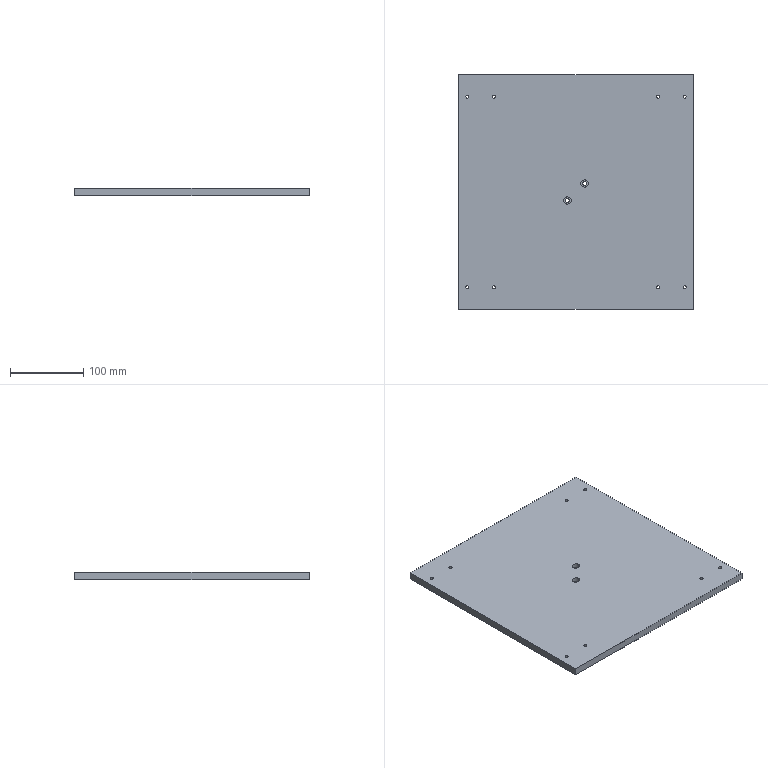Part | SolidWorks | features HoleWzd 2, MirrorPattern 2, Extrusion 1 | 1 solid | 32 faces | box 320 x 320 x 10 mm | volume 1021792 mm3 | cylinder 24 | plane 8 | commonest cylinder face diameters 4.2 x16 5.5 x4 10 x4
STEP:
#1=CARTESIAN_POINT('',(-145.9,-130.,10.));
#2=VERTEX_POINT('',#1);
#3=CARTESIAN_POINT('',(-150.1,-130.,10.));
#4=VERTEX_POINT('',#3);
#5=CARTESIAN_POINT('',(-148.,-130.,10.));
#6=DIRECTION('',(0.,0.,-1.));
#7=DIRECTION('',(-1.,0.,0.));
#8=AXIS2_PLACEMENT_3D('',#5,#6,#7);
#9=CIRCLE('',#8,2.1);
#10=EDGE_CURVE('',#2,#4,#9,.T.);
#11=ORIENTED_EDGE('',*,*,#10,.F.);
#12=CARTESIAN_POINT('',(-145.9,-130.,0.));
#13=VERTEX_POINT('',#12);
#14=CARTESIAN_POINT('',(-145.9,-130.,0.));
#15=DIRECTION('',(0.,0.,-1.));
#16=VECTOR('',#15,1000.);
#17=LINE('',#14,#16);
#18=EDGE_CURVE('',#2,#13,#17,.T.);
#19=ORIENTED_EDGE('',*,*,#18,.T.);
#20=CARTESIAN_POINT('',(-150.1,-130.,0.));
#21=VERTEX_POINT('',#20);
#22=CARTESIAN_POINT('',(-148.,-130.,0.));
#23=DIRECTION('',(0.,0.,-1.));
#24=DIRECTION('',(-1.,0.,0.));
#25=AXIS2_PLACEMENT_3D('',#22,#23,#24);
#26=CIRCLE('',#25,2.1);
#27=EDGE_CURVE('',#13,#21,#26,.T.);
#28=ORIENTED_EDGE('',*,*,#27,.T.);
#29=CARTESIAN_POINT('',(-150.1,-130.,0.));
#30=DIRECTION('',(0.,0.,-1.));
#31=VECTOR('',#30,1000.);
#32=LINE('',#29,#31);
#33=EDGE_CURVE('',#4,#21,#32,.T.);
#34=ORIENTED_EDGE('',*,*,#33,.F.);
#35=EDGE_LOOP('',(#11,#19,#28,#34));
#36=FACE_OUTER_BOUND('',#35,.T.);
#37=CARTESIAN_POINT('',(-148.,-130.,0.));
#38=DIRECTION('',(0.,0.,-1.));
#39=DIRECTION('',(-1.,0.,0.));
#40=AXIS2_PLACEMENT_3D('',#37,#38,#39);
#41=CYLINDRICAL_SURFACE('',#40,2.1);
#42=ADVANCED_FACE('',(#36),#41,.F.);
#43=CARTESIAN_POINT('',(-109.9,-130.,10.));
#44=VERTEX_POINT('',#43);
#45=CARTESIAN_POINT('',(-114.1,-130.,10.));
#46=VERTEX_POINT('',#45);
#47=CARTESIAN_POINT('',(-112.,-130.,10.));
#48=DIRECTION('',(0.,0.,-1.));
#49=DIRECTION('',(-1.,0.,0.));
#50=AXIS2_PLACEMENT_3D('',#47,#48,#49);
#51=CIRCLE('',#50,2.1);
#52=EDGE_CURVE('',#44,#46,#51,.T.);
#53=ORIENTED_EDGE('',*,*,#52,.F.);
#54=CARTESIAN_POINT('',(-109.9,-130.,0.));
#55=VERTEX_POINT('',#54);
#56=CARTESIAN_POINT('',(-109.9,-130.,0.));
#57=DIRECTION('',(0.,0.,-1.));
#58=VECTOR('',#57,1000.);
#59=LINE('',#56,#58);
#60=EDGE_CURVE('',#44,#55,#59,.T.);
#61=ORIENTED_EDGE('',*,*,#60,.T.);
#62=CARTESIAN_POINT('',(-114.1,-130.,0.));
#63=VERTEX_POINT('',#62);
#64=CARTESIAN_POINT('',(-112.,-130.,0.));
#65=DIRECTION('',(0.,0.,-1.));
#66=DIRECTION('',(-1.,0.,0.));
#67=AXIS2_PLACEMENT_3D('',#64,#65,#66);
#68=CIRCLE('',#67,2.1);
#69=EDGE_CURVE('',#55,#63,#68,.T.);
#70=ORIENTED_EDGE('',*,*,#69,.T.);
#71=CARTESIAN_POINT('',(-114.1,-130.,0.));
#72=DIRECTION('',(0.,0.,-1.));
#73=VECTOR('',#72,1000.);
#74=LINE('',#71,#73);
#75=EDGE_CURVE('',#46,#63,#74,.T.);
#76=ORIENTED_EDGE('',*,*,#75,.F.);
#77=EDGE_LOOP('',(#53,#61,#70,#76));
#78=FACE_OUTER_BOUND('',#77,.T.);
#79=CARTESIAN_POINT('',(-112.,-130.,0.));
#80=DIRECTION('',(0.,0.,-1.));
#81=DIRECTION('',(-1.,0.,0.));
#82=AXIS2_PLACEMENT_3D('',#79,#80,#81);
#83=CYLINDRICAL_SURFACE('',#82,2.1);
#84=ADVANCED_FACE('',(#78),#83,.F.);
#85=CARTESIAN_POINT('',(-145.9,130.,10.));
#86=VERTEX_POINT('',#85);
#87=CARTESIAN_POINT('',(-150.1,130.,10.));
#88=VERTEX_POINT('',#87);
#89=CARTESIAN_POINT('',(-148.,130.,10.));
#90=DIRECTION('',(0.,0.,-1.));
#91=DIRECTION('',(-1.,0.,0.));
#92=AXIS2_PLACEMENT_3D('',#89,#90,#91);
#93=CIRCLE('',#92,2.1);
#94=EDGE_CURVE('',#86,#88,#93,.T.);
#95=ORIENTED_EDGE('',*,*,#94,.F.);
#96=CARTESIAN_POINT('',(-145.9,130.,0.));
#97=VERTEX_POINT('',#96);
#98=CARTESIAN_POINT('',(-145.9,130.,0.));
#99=DIRECTION('',(0.,0.,-1.));
#100=VECTOR('',#99,1000.);
#101=LINE('',#98,#100);
#102=EDGE_CURVE('',#86,#97,#101,.T.);
#103=ORIENTED_EDGE('',*,*,#102,.T.);
#104=CARTESIAN_POINT('',(-150.1,130.,0.));
#105=VERTEX_POINT('',#104);
#106=CARTESIAN_POINT('',(-148.,130.,0.));
#107=DIRECTION('',(0.,0.,-1.));
#108=DIRECTION('',(-1.,0.,0.));
#109=AXIS2_PLACEMENT_3D('',#106,#107,#108);
#110=CIRCLE('',#109,2.1);
#111=EDGE_CURVE('',#97,#105,#110,.T.);
#112=ORIENTED_EDGE('',*,*,#111,.T.);
#113=CARTESIAN_POINT('',(-150.1,130.,0.));
#114=DIRECTION('',(0.,0.,-1.));
#115=VECTOR('',#114,1000.);
#116=LINE('',#113,#115);
#117=EDGE_CURVE('',#88,#105,#116,.T.);
#118=ORIENTED_EDGE('',*,*,#117,.F.);
#119=EDGE_LOOP('',(#95,#103,#112,#118));
#120=FACE_OUTER_BOUND('',#119,.T.);
#121=CARTESIAN_POINT('',(-148.,130.,0.));
#122=DIRECTION('',(0.,0.,-1.));
#123=DIRECTION('',(-1.,0.,0.));
#124=AXIS2_PLACEMENT_3D('',#121,#122,#123);
#125=CYLINDRICAL_SURFACE('',#124,2.1);
#126=ADVANCED_FACE('',(#120),#125,.F.);
#127=CARTESIAN_POINT('',(-109.9,130.,10.));
#128=VERTEX_POINT('',#127);
#129=CARTESIAN_POINT('',(-114.1,130.,10.));
#130=VERTEX_POINT('',#129);
#131=CARTESIAN_POINT('',(-112.,130.,10.));
#132=DIRECTION('',(0.,0.,-1.));
#133=DIRECTION('',(-1.,0.,0.));
#134=AXIS2_PLACEMENT_3D('',#131,#132,#133);
#135=CIRCLE('',#134,2.1);
#136=EDGE_CURVE('',#128,#130,#135,.T.);
#137=ORIENTED_EDGE('',*,*,#136,.F.);
#138=CARTESIAN_POINT('',(-109.9,130.,0.));
#139=VERTEX_POINT('',#138);
#140=CARTESIAN_POINT('',(-109.9,130.,0.));
#141=DIRECTION('',(0.,0.,-1.));
#142=VECTOR('',#141,1000.);
#143=LINE('',#140,#142);
#144=EDGE_CURVE('',#128,#139,#143,.T.);
#145=ORIENTED_EDGE('',*,*,#144,.T.);
#146=CARTESIAN_POINT('',(-114.1,130.,0.));
#147=VERTEX_POINT('',#146);
#148=CARTESIAN_POINT('',(-112.,130.,0.));
#149=DIRECTION('',(0.,0.,-1.));
#150=DIRECTION('',(-1.,0.,0.));
#151=AXIS2_PLACEMENT_3D('',#148,#149,#150);
#152=CIRCLE('',#151,2.1);
#153=EDGE_CURVE('',#139,#147,#152,.T.);
#154=ORIENTED_EDGE('',*,*,#153,.T.);
#155=CARTESIAN_POINT('',(-114.1,130.,0.));
#156=DIRECTION('',(0.,0.,-1.));
#157=VECTOR('',#156,1000.);
#158=LINE('',#155,#157);
#159=EDGE_CURVE('',#130,#147,#158,.T.);
#160=ORIENTED_EDGE('',*,*,#159,.F.);
#161=EDGE_LOOP('',(#137,#145,#154,#160));
#162=FACE_OUTER_BOUND('',#161,.T.);
#163=CARTESIAN_POINT('',(-112.,130.,0.));
#164=DIRECTION('',(0.,0.,-1.));
#165=DIRECTION('',(-1.,0.,0.));
#166=AXIS2_PLACEMENT_3D('',#163,#164,#165);
#167=CYLINDRICAL_SURFACE('',#166,2.1);
#168=ADVANCED_FACE('',(#162),#167,.F.);
#169=CARTESIAN_POINT('',(150.1,-130.,10.));
#170=VERTEX_POINT('',#169);
#171=CARTESIAN_POINT('',(145.9,-130.,10.));
#172=VERTEX_POINT('',#171);
#173=CARTESIAN_POINT('',(148.,-130.,10.));
#174=DIRECTION('',(0.,0.,-1.));
#175=DIRECTION('',(-1.,0.,0.));
#176=AXIS2_PLACEMENT_3D('',#173,#174,#175);
#177=CIRCLE('',#176,2.1);
#178=EDGE_CURVE('',#170,#172,#177,.T.);
#179=ORIENTED_EDGE('',*,*,#178,.F.);
#180=CARTESIAN_POINT('',(150.1,-130.,0.));
#181=VERTEX_POINT('',#180);
#182=CARTESIAN_POINT('',(150.1,-130.,0.));
#183=DIRECTION('',(0.,0.,-1.));
#184=VECTOR('',#183,1000.);
#185=LINE('',#182,#184);
#186=EDGE_CURVE('',#170,#181,#185,.T.);
#187=ORIENTED_EDGE('',*,*,#186,.T.);
#188=CARTESIAN_POINT('',(145.9,-130.,0.));
#189=VERTEX_POINT('',#188);
#190=CARTESIAN_POINT('',(148.,-130.,0.));
#191=DIRECTION('',(0.,0.,-1.));
#192=DIRECTION('',(-1.,0.,0.));
#193=AXIS2_PLACEMENT_3D('',#190,#191,#192);
#194=CIRCLE('',#193,2.1);
#195=EDGE_CURVE('',#181,#189,#194,.T.);
#196=ORIENTED_EDGE('',*,*,#195,.T.);
#197=CARTESIAN_POINT('',(145.9,-130.,0.));
#198=DIRECTION('',(0.,0.,-1.));
#199=VECTOR('',#198,1000.);
#200=LINE('',#197,#199);
#201=EDGE_CURVE('',#172,#189,#200,.T.);
#202=ORIENTED_EDGE('',*,*,#201,.F.);
#203=EDGE_LOOP('',(#179,#187,#196,#202));
#204=FACE_OUTER_BOUND('',#203,.T.);
#205=CARTESIAN_POINT('',(148.,-130.,0.));
#206=DIRECTION('',(0.,0.,-1.));
#207=DIRECTION('',(-1.,0.,0.));
#208=AXIS2_PLACEMENT_3D('',#205,#206,#207);
#209=CYLINDRICAL_SURFACE('',#208,2.1);
#210=ADVANCED_FACE('',(#204),#209,.F.);
#211=CARTESIAN_POINT('',(114.1,-130.,10.));
#212=VERTEX_POINT('',#211);
#213=CARTESIAN_POINT('',(109.9,-130.,10.));
#214=VERTEX_POINT('',#213);
#215=CARTESIAN_POINT('',(112.,-130.,10.));
#216=DIRECTION('',(0.,0.,-1.));
#217=DIRECTION('',(-1.,0.,0.));
#218=AXIS2_PLACEMENT_3D('',#215,#216,#217);
#219=CIRCLE('',#218,2.1);
#220=EDGE_CURVE('',#212,#214,#219,.T.);
#221=ORIENTED_EDGE('',*,*,#220,.F.);
#222=CARTESIAN_POINT('',(114.1,-130.,0.));
#223=VERTEX_POINT('',#222);
#224=CARTESIAN_POINT('',(114.1,-130.,0.));
#225=DIRECTION('',(0.,0.,-1.));
#226=VECTOR('',#225,1000.);
#227=LINE('',#224,#226);
#228=EDGE_CURVE('',#212,#223,#227,.T.);
#229=ORIENTED_EDGE('',*,*,#228,.T.);
#230=CARTESIAN_POINT('',(109.9,-130.,0.));
#231=VERTEX_POINT('',#230);
#232=CARTESIAN_POINT('',(112.,-130.,0.));
#233=DIRECTION('',(0.,0.,-1.));
#234=DIRECTION('',(-1.,0.,0.));
#235=AXIS2_PLACEMENT_3D('',#232,#233,#234);
#236=CIRCLE('',#235,2.1);
#237=EDGE_CURVE('',#223,#231,#236,.T.);
#238=ORIENTED_EDGE('',*,*,#237,.T.);
#239=CARTESIAN_POINT('',(109.9,-130.,0.));
#240=DIRECTION('',(0.,0.,-1.));
#241=VECTOR('',#240,1000.);
#242=LINE('',#239,#241);
#243=EDGE_CURVE('',#214,#231,#242,.T.);
#244=ORIENTED_EDGE('',*,*,#243,.F.);
#245=EDGE_LOOP('',(#221,#229,#238,#244));
#246=FACE_OUTER_BOUND('',#245,.T.);
#247=CARTESIAN_POINT('',(112.,-130.,0.));
#248=DIRECTION('',(0.,0.,-1.));
#249=DIRECTION('',(-1.,0.,0.));
#250=AXIS2_PLACEMENT_3D('',#247,#248,#249);
#251=CYLINDRICAL_SURFACE('',#250,2.1);
#252=ADVANCED_FACE('',(#246),#251,.F.);
#253=CARTESIAN_POINT('',(150.1,130.,10.));
#254=VERTEX_POINT('',#253);
#255=CARTESIAN_POINT('',(145.9,130.,10.));
#256=VERTEX_POINT('',#255);
#257=CARTESIAN_POINT('',(148.,130.,10.));
#258=DIRECTION('',(0.,0.,-1.));
#259=DIRECTION('',(-1.,0.,0.));
#260=AXIS2_PLACEMENT_3D('',#257,#258,#259);
#261=CIRCLE('',#260,2.1);
#262=EDGE_CURVE('',#254,#256,#261,.T.);
#263=ORIENTED_EDGE('',*,*,#262,.F.);
#264=CARTESIAN_POINT('',(150.1,130.,0.));
#265=VERTEX_POINT('',#264);
#266=CARTESIAN_POINT('',(150.1,130.,0.));
#267=DIRECTION('',(0.,0.,-1.));
#268=VECTOR('',#267,1000.);
#269=LINE('',#266,#268);
#270=EDGE_CURVE('',#254,#265,#269,.T.);
#271=ORIENTED_EDGE('',*,*,#270,.T.);
#272=CARTESIAN_POINT('',(145.9,130.,0.));
#273=VERTEX_POINT('',#272);
#274=CARTESIAN_POINT('',(148.,130.,0.));
#275=DIRECTION('',(0.,0.,-1.));
#276=DIRECTION('',(-1.,0.,0.));
#277=AXIS2_PLACEMENT_3D('',#274,#275,#276);
#278=CIRCLE('',#277,2.1);
#279=EDGE_CURVE('',#265,#273,#278,.T.);
#280=ORIENTED_EDGE('',*,*,#279,.T.);
#281=CARTESIAN_POINT('',(145.9,130.,0.));
#282=DIRECTION('',(0.,0.,-1.));
#283=VECTOR('',#282,1000.);
#284=LINE('',#281,#283);
#285=EDGE_CURVE('',#256,#273,#284,.T.);
#286=ORIENTED_EDGE('',*,*,#285,.F.);
#287=EDGE_LOOP('',(#263,#271,#280,#286));
#288=FACE_OUTER_BOUND('',#287,.T.);
#289=CARTESIAN_POINT('',(148.,130.,0.));
#290=DIRECTION('',(0.,0.,-1.));
#291=DIRECTION('',(-1.,0.,0.));
#292=AXIS2_PLACEMENT_3D('',#289,#290,#291);
#293=CYLINDRICAL_SURFACE('',#292,2.1);
#294=ADVANCED_FACE('',(#288),#293,.F.);
#295=CARTESIAN_POINT('',(114.1,130.,10.));
#296=VERTEX_POINT('',#295);
#297=CARTESIAN_POINT('',(109.9,130.,10.));
#298=VERTEX_POINT('',#297);
#299=CARTESIAN_POINT('',(112.,130.,10.));
#300=DIRECTION('',(0.,0.,-1.));
#301=DIRECTION('',(-1.,0.,0.));
#302=AXIS2_PLACEMENT_3D('',#299,#300,#301);
#303=CIRCLE('',#302,2.1);
#304=EDGE_CURVE('',#296,#298,#303,.T.);
#305=ORIENTED_EDGE('',*,*,#304,.F.);
#306=CARTESIAN_POINT('',(114.1,130.,0.));
#307=VERTEX_POINT('',#306);
#308=CARTESIAN_POINT('',(114.1,130.,0.));
#309=DIRECTION('',(0.,0.,-1.));
#310=VECTOR('',#309,1000.);
#311=LINE('',#308,#310);
#312=EDGE_CURVE('',#296,#307,#311,.T.);
#313=ORIENTED_EDGE('',*,*,#312,.T.);
#314=CARTESIAN_POINT('',(109.9,130.,0.));
#315=VERTEX_POINT('',#314);
#316=CARTESIAN_POINT('',(112.,130.,0.));
#317=DIRECTION('',(0.,0.,-1.));
#318=DIRECTION('',(-1.,0.,0.));
#319=AXIS2_PLACEMENT_3D('',#316,#317,#318);
#320=CIRCLE('',#319,2.1);
#321=EDGE_CURVE('',#307,#315,#320,.T.);
#322=ORIENTED_EDGE('',*,*,#321,.T.);
#323=CARTESIAN_POINT('',(109.9,130.,0.));
#324=DIRECTION('',(0.,0.,-1.));
#325=VECTOR('',#324,1000.);
#326=LINE('',#323,#325);
#327=EDGE_CURVE('',#298,#315,#326,.T.);
#328=ORIENTED_EDGE('',*,*,#327,.F.);
#329=EDGE_LOOP('',(#305,#313,#322,#328));
#330=FACE_OUTER_BOUND('',#329,.T.);
#331=CARTESIAN_POINT('',(112.,130.,0.));
#332=DIRECTION('',(0.,0.,-1.));
#333=DIRECTION('',(-1.,0.,0.));
#334=AXIS2_PLACEMENT_3D('',#331,#332,#333);
#335=CYLINDRICAL_SURFACE('',#334,2.1);
#336=ADVANCED_FACE('',(#330),#335,.F.);
#337=CARTESIAN_POINT('',(-16.667,-11.667,4.3));
#338=VERTEX_POINT('',#337);
#339=CARTESIAN_POINT('',(-6.667,-11.667,4.3));
#340=VERTEX_POINT('',#339);
#341=CARTESIAN_POINT('',(-11.667,-11.667,4.3));
#342=DIRECTION('',(0.,0.,1.));
#343=DIRECTION('',(1.,0.,0.));
#344=AXIS2_PLACEMENT_3D('',#341,#342,#343);
#345=CIRCLE('',#344,5.);
#346=EDGE_CURVE('',#338,#340,#345,.T.);
#347=ORIENTED_EDGE('',*,*,#346,.F.);
#348=CARTESIAN_POINT('',(-16.667,-11.667,10.));
#349=VERTEX_POINT('',#348);
#350=CARTESIAN_POINT('',(-16.667,-11.667,10.));
#351=DIRECTION('',(0.,0.,1.));
#352=VECTOR('',#351,1000.);
#353=LINE('',#350,#352);
#354=EDGE_CURVE('',#338,#349,#353,.T.);
#355=ORIENTED_EDGE('',*,*,#354,.T.);
#356=CARTESIAN_POINT('',(-6.667,-11.667,10.));
#357=VERTEX_POINT('',#356);
#358=CARTESIAN_POINT('',(-11.667,-11.667,10.));
#359=DIRECTION('',(0.,0.,1.));
#360=DIRECTION('',(1.,0.,0.));
#361=AXIS2_PLACEMENT_3D('',#358,#359,#360);
#362=CIRCLE('',#361,5.);
#363=EDGE_CURVE('',#349,#357,#362,.T.);
#364=ORIENTED_EDGE('',*,*,#363,.T.);
#365=CARTESIAN_POINT('',(-6.667,-11.667,10.));
#366=DIRECTION('',(0.,0.,1.));
#367=VECTOR('',#366,1000.);
#368=LINE('',#365,#367);
#369=EDGE_CURVE('',#340,#357,#368,.T.);
#370=ORIENTED_EDGE('',*,*,#369,.F.);
#371=EDGE_LOOP('',(#347,#355,#364,#370));
#372=FACE_OUTER_BOUND('',#371,.T.);
#373=CARTESIAN_POINT('',(-11.667,-11.667,10.));
#374=DIRECTION('',(0.,0.,1.));
#375=DIRECTION('',(1.,0.,0.));
#376=AXIS2_PLACEMENT_3D('',#373,#374,#375);
#377=CYLINDRICAL_SURFACE('',#376,5.);
#378=ADVANCED_FACE('',(#372),#377,.F.);
#379=CARTESIAN_POINT('',(-14.417,-11.667,0.));
#380=VERTEX_POINT('',#379);
#381=CARTESIAN_POINT('',(-8.917,-11.667,0.));
#382=VERTEX_POINT('',#381);
#383=CARTESIAN_POINT('',(-11.667,-11.667,0.));
#384=DIRECTION('',(0.,0.,1.));
#385=DIRECTION('',(1.,0.,0.));
#386=AXIS2_PLACEMENT_3D('',#383,#384,#385);
#387=CIRCLE('',#386,2.75);
#388=EDGE_CURVE('',#380,#382,#387,.T.);
#389=ORIENTED_EDGE('',*,*,#388,.F.);
#390=CARTESIAN_POINT('',(-14.417,-11.667,4.3));
#391=VERTEX_POINT('',#390);
#392=CARTESIAN_POINT('',(-14.417,-11.667,10.));
#393=DIRECTION('',(0.,0.,1.));
#394=VECTOR('',#393,1000.);
#395=LINE('',#392,#394);
#396=EDGE_CURVE('',#380,#391,#395,.T.);
#397=ORIENTED_EDGE('',*,*,#396,.T.);
#398=CARTESIAN_POINT('',(-8.917,-11.667,4.3));
#399=VERTEX_POINT('',#398);
#400=CARTESIAN_POINT('',(-11.667,-11.667,4.3));
#401=DIRECTION('',(0.,0.,1.));
#402=DIRECTION('',(1.,0.,0.));
#403=AXIS2_PLACEMENT_3D('',#400,#401,#402);
#404=CIRCLE('',#403,2.75);
#405=EDGE_CURVE('',#391,#399,#404,.T.);
#406=ORIENTED_EDGE('',*,*,#405,.T.);
#407=CARTESIAN_POINT('',(-8.917,-11.667,10.));
#408=DIRECTION('',(0.,0.,1.));
#409=VECTOR('',#408,1000.);
#410=LINE('',#407,#409);
#411=EDGE_CURVE('',#382,#399,#410,.T.);
#412=ORIENTED_EDGE('',*,*,#411,.F.);
#413=EDGE_LOOP('',(#389,#397,#406,#412));
#414=FACE_OUTER_BOUND('',#413,.T.);
#415=CARTESIAN_POINT('',(-11.667,-11.667,10.));
#416=DIRECTION('',(0.,0.,1.));
#417=DIRECTION('',(1.,0.,0.));
#418=AXIS2_PLACEMENT_3D('',#415,#416,#417);
#419=CYLINDRICAL_SURFACE('',#418,2.75);
#420=ADVANCED_FACE('',(#414),#419,.F.);
#421=CARTESIAN_POINT('',(6.667,11.667,4.3));
#422=VERTEX_POINT('',#421);
#423=CARTESIAN_POINT('',(16.667,11.667,4.3));
#424=VERTEX_POINT('',#423);
#425=CARTESIAN_POINT('',(11.667,11.667,4.3));
#426=DIRECTION('',(0.,0.,1.));
#427=DIRECTION('',(1.,0.,0.));
#428=AXIS2_PLACEMENT_3D('',#425,#426,#427);
#429=CIRCLE('',#428,5.);
#430=EDGE_CURVE('',#422,#424,#429,.T.);
#431=ORIENTED_EDGE('',*,*,#430,.F.);
#432=CARTESIAN_POINT('',(6.667,11.667,10.));
#433=VERTEX_POINT('',#432);
#434=CARTESIAN_POINT('',(6.667,11.667,10.));
#435=DIRECTION('',(0.,0.,1.));
#436=VECTOR('',#435,1000.);
#437=LINE('',#434,#436);
#438=EDGE_CURVE('',#422,#433,#437,.T.);
#439=ORIENTED_EDGE('',*,*,#438,.T.);
#440=CARTESIAN_POINT('',(16.667,11.667,10.));
#441=VERTEX_POINT('',#440);
#442=CARTESIAN_POINT('',(11.667,11.667,10.));
#443=DIRECTION('',(0.,0.,1.));
#444=DIRECTION('',(1.,0.,0.));
#445=AXIS2_PLACEMENT_3D('',#442,#443,#444);
#446=CIRCLE('',#445,5.);
#447=EDGE_CURVE('',#433,#441,#446,.T.);
#448=ORIENTED_EDGE('',*,*,#447,.T.);
#449=CARTESIAN_POINT('',(16.667,11.667,10.));
#450=DIRECTION('',(0.,0.,1.));
#451=VECTOR('',#450,1000.);
#452=LINE('',#449,#451);
#453=EDGE_CURVE('',#424,#441,#452,.T.);
#454=ORIENTED_EDGE('',*,*,#453,.F.);
#455=EDGE_LOOP('',(#431,#439,#448,#454));
#456=FACE_OUTER_BOUND('',#455,.T.);
#457=CARTESIAN_POINT('',(11.667,11.667,10.));
#458=DIRECTION('',(0.,0.,1.));
#459=DIRECTION('',(1.,0.,0.));
#460=AXIS2_PLACEMENT_3D('',#457,#458,#459);
#461=CYLINDRICAL_SURFACE('',#460,5.);
#462=ADVANCED_FACE('',(#456),#461,.F.);
#463=CARTESIAN_POINT('',(8.917,11.667,0.));
#464=VERTEX_POINT('',#463);
#465=CARTESIAN_POINT('',(14.417,11.667,0.));
#466=VERTEX_POINT('',#465);
#467=CARTESIAN_POINT('',(11.667,11.667,0.));
#468=DIRECTION('',(0.,0.,1.));
#469=DIRECTION('',(1.,0.,0.));
#470=AXIS2_PLACEMENT_3D('',#467,#468,#469);
#471=CIRCLE('',#470,2.75);
#472=EDGE_CURVE('',#464,#466,#471,.T.);
#473=ORIENTED_EDGE('',*,*,#472,.F.);
#474=CARTESIAN_POINT('',(8.917,11.667,4.3));
#475=VERTEX_POINT('',#474);
#476=CARTESIAN_POINT('',(8.917,11.667,10.));
#477=DIRECTION('',(0.,0.,1.));
#478=VECTOR('',#477,1000.);
#479=LINE('',#476,#478);
#480=EDGE_CURVE('',#464,#475,#479,.T.);
#481=ORIENTED_EDGE('',*,*,#480,.T.);
#482=CARTESIAN_POINT('',(14.417,11.667,4.3));
#483=VERTEX_POINT('',#482);
#484=CARTESIAN_POINT('',(11.667,11.667,4.3));
#485=DIRECTION('',(0.,0.,1.));
#486=DIRECTION('',(1.,0.,0.));
#487=AXIS2_PLACEMENT_3D('',#484,#485,#486);
#488=CIRCLE('',#487,2.75);
#489=EDGE_CURVE('',#475,#483,#488,.T.);
#490=ORIENTED_EDGE('',*,*,#489,.T.);
#491=CARTESIAN_POINT('',(14.417,11.667,10.));
#492=DIRECTION('',(0.,0.,1.));
#493=VECTOR('',#492,1000.);
#494=LINE('',#491,#493);
#495=EDGE_CURVE('',#466,#483,#494,.T.);
#496=ORIENTED_EDGE('',*,*,#495,.F.);
#497=EDGE_LOOP('',(#473,#481,#490,#496));
#498=FACE_OUTER_BOUND('',#497,.T.);
#499=CARTESIAN_POINT('',(11.667,11.667,10.));
#500=DIRECTION('',(0.,0.,1.));
#501=DIRECTION('',(1.,0.,0.));
#502=AXIS2_PLACEMENT_3D('',#499,#500,#501);
#503=CYLINDRICAL_SURFACE('',#502,2.75);
#504=ADVANCED_FACE('',(#498),#503,.F.);
#505=CARTESIAN_POINT('',(-148.,130.,10.));
#506=DIRECTION('',(0.,0.,-1.));
#507=DIRECTION('',(-1.,0.,0.));
#508=AXIS2_PLACEMENT_3D('',#505,#506,#507);
#509=CIRCLE('',#508,2.1);
#510=EDGE_CURVE('',#88,#86,#509,.T.);
#511=ORIENTED_EDGE('',*,*,#510,.T.);
#512=ORIENTED_EDGE('',*,*,#94,.T.);
#513=EDGE_LOOP('',(#511,#512));
#514=FACE_BOUND('',#513,.T.);
#515=CARTESIAN_POINT('',(-112.,130.,10.));
#516=DIRECTION('',(0.,0.,-1.));
#517=DIRECTION('',(-1.,0.,0.));
#518=AXIS2_PLACEMENT_3D('',#515,#516,#517);
#519=CIRCLE('',#518,2.1);
#520=EDGE_CURVE('',#130,#128,#519,.T.);
#521=ORIENTED_EDGE('',*,*,#520,.T.);
#522=ORIENTED_EDGE('',*,*,#136,.T.);
#523=EDGE_LOOP('',(#521,#522));
#524=FACE_BOUND('',#523,.T.);
#525=CARTESIAN_POINT('',(160.,-160.,10.));
#526=VERTEX_POINT('',#525);
#527=CARTESIAN_POINT('',(160.,160.,10.));
#528=VERTEX_POINT('',#527);
#529=CARTESIAN_POINT('',(160.,160.,10.));
#530=DIRECTION('',(0.,1.,0.));
#531=VECTOR('',#530,1000.);
#532=LINE('',#529,#531);
#533=EDGE_CURVE('',#526,#528,#532,.T.);
#534=ORIENTED_EDGE('',*,*,#533,.T.);
#535=CARTESIAN_POINT('',(-160.,160.,10.));
#536=VERTEX_POINT('',#535);
#537=CARTESIAN_POINT('',(-160.,160.,10.));
#538=DIRECTION('',(-1.,0.,0.));
#539=VECTOR('',#538,1000.);
#540=LINE('',#537,#539);
#541=EDGE_CURVE('',#528,#536,#540,.T.);
#542=ORIENTED_EDGE('',*,*,#541,.T.);
#543=CARTESIAN_POINT('',(-160.,-160.,10.));
#544=VERTEX_POINT('',#543);
#545=CARTESIAN_POINT('',(-160.,160.,10.));
#546=DIRECTION('',(0.,-1.,0.));
#547=VECTOR('',#546,1000.);
#548=LINE('',#545,#547);
#549=EDGE_CURVE('',#536,#544,#548,.T.);
#550=ORIENTED_EDGE('',*,*,#549,.T.);
#551=CARTESIAN_POINT('',(-160.,-160.,10.));
#552=DIRECTION('',(1.,0.,0.));
#553=VECTOR('',#552,1000.);
#554=LINE('',#551,#553);
#555=EDGE_CURVE('',#544,#526,#554,.T.);
#556=ORIENTED_EDGE('',*,*,#555,.T.);
#557=EDGE_LOOP('',(#534,#542,#550,#556));
#558=FACE_OUTER_BOUND('',#557,.T.);
#559=CARTESIAN_POINT('',(11.667,11.667,10.));
#560=DIRECTION('',(0.,0.,1.));
#561=DIRECTION('',(1.,0.,0.));
#562=AXIS2_PLACEMENT_3D('',#559,#560,#561);
#563=CIRCLE('',#562,5.);
#564=EDGE_CURVE('',#441,#433,#563,.T.);
#565=ORIENTED_EDGE('',*,*,#564,.F.);
#566=ORIENTED_EDGE('',*,*,#447,.F.);
#567=EDGE_LOOP('',(#565,#566));
#568=FACE_BOUND('',#567,.T.);
#569=CARTESIAN_POINT('',(-11.667,-11.667,10.));
#570=DIRECTION('',(0.,0.,1.));
#571=DIRECTION('',(1.,0.,0.));
#572=AXIS2_PLACEMENT_3D('',#569,#570,#571);
#573=CIRCLE('',#572,5.);
#574=EDGE_CURVE('',#357,#349,#573,.T.);
#575=ORIENTED_EDGE('',*,*,#574,.F.);
#576=ORIENTED_EDGE('',*,*,#363,.F.);
#577=EDGE_LOOP('',(#575,#576));
#578=FACE_BOUND('',#577,.T.);
#579=CARTESIAN_POINT('',(112.,130.,10.));
#580=DIRECTION('',(0.,0.,-1.));
#581=DIRECTION('',(-1.,0.,0.));
#582=AXIS2_PLACEMENT_3D('',#579,#580,#581);
#583=CIRCLE('',#582,2.1);
#584=EDGE_CURVE('',#298,#296,#583,.T.);
#585=ORIENTED_EDGE('',*,*,#584,.T.);
#586=ORIENTED_EDGE('',*,*,#304,.T.);
#587=EDGE_LOOP('',(#585,#586));
#588=FACE_BOUND('',#587,.T.);
#589=CARTESIAN_POINT('',(148.,130.,10.));
#590=DIRECTION('',(0.,0.,-1.));
#591=DIRECTION('',(-1.,0.,0.));
#592=AXIS2_PLACEMENT_3D('',#589,#590,#591);
#593=CIRCLE('',#592,2.1);
#594=EDGE_CURVE('',#256,#254,#593,.T.);
#595=ORIENTED_EDGE('',*,*,#594,.T.);
#596=ORIENTED_EDGE('',*,*,#262,.T.);
#597=EDGE_LOOP('',(#595,#596));
#598=FACE_BOUND('',#597,.T.);
#599=CARTESIAN_POINT('',(112.,-130.,10.));
#600=DIRECTION('',(0.,0.,-1.));
#601=DIRECTION('',(-1.,0.,0.));
#602=AXIS2_PLACEMENT_3D('',#599,#600,#601);
#603=CIRCLE('',#602,2.1);
#604=EDGE_CURVE('',#214,#212,#603,.T.);
#605=ORIENTED_EDGE('',*,*,#604,.T.);
#606=ORIENTED_EDGE('',*,*,#220,.T.);
#607=EDGE_LOOP('',(#605,#606));
#608=FACE_BOUND('',#607,.T.);
#609=CARTESIAN_POINT('',(148.,-130.,10.));
#610=DIRECTION('',(0.,0.,-1.));
#611=DIRECTION('',(-1.,0.,0.));
#612=AXIS2_PLACEMENT_3D('',#609,#610,#611);
#613=CIRCLE('',#612,2.1);
#614=EDGE_CURVE('',#172,#170,#613,.T.);
#615=ORIENTED_EDGE('',*,*,#614,.T.);
#616=ORIENTED_EDGE('',*,*,#178,.T.);
#617=EDGE_LOOP('',(#615,#616));
#618=FACE_BOUND('',#617,.T.);
#619=CARTESIAN_POINT('',(-112.,-130.,10.));
#620=DIRECTION('',(0.,0.,-1.));
#621=DIRECTION('',(-1.,0.,0.));
#622=AXIS2_PLACEMENT_3D('',#619,#620,#621);
#623=CIRCLE('',#622,2.1);
#624=EDGE_CURVE('',#46,#44,#623,.T.);
#625=ORIENTED_EDGE('',*,*,#624,.T.);
#626=ORIENTED_EDGE('',*,*,#52,.T.);
#627=EDGE_LOOP('',(#625,#626));
#628=FACE_BOUND('',#627,.T.);
#629=CARTESIAN_POINT('',(-148.,-130.,10.));
#630=DIRECTION('',(0.,0.,-1.));
#631=DIRECTION('',(-1.,0.,0.));
#632=AXIS2_PLACEMENT_3D('',#629,#630,#631);
#633=CIRCLE('',#632,2.1);
#634=EDGE_CURVE('',#4,#2,#633,.T.);
#635=ORIENTED_EDGE('',*,*,#634,.T.);
#636=ORIENTED_EDGE('',*,*,#10,.T.);
#637=EDGE_LOOP('',(#635,#636));
#638=FACE_BOUND('',#637,.T.);
#639=CARTESIAN_POINT('',(0.,0.,10.));
#640=DIRECTION('',(0.,0.,1.));
#641=DIRECTION('',(1.,0.,0.));
#642=AXIS2_PLACEMENT_3D('',#639,#640,#641);
#643=PLANE('',#642);
#644=ADVANCED_FACE('',(#514,#524,#558,#568,#578,#588,#598,#608,#618,#628,#638),#643,.T.);
#645=CARTESIAN_POINT('',(-148.,130.,0.));
#646=DIRECTION('',(0.,0.,-1.));
#647=DIRECTION('',(-1.,0.,0.));
#648=AXIS2_PLACEMENT_3D('',#645,#646,#647);
#649=CIRCLE('',#648,2.1);
#650=EDGE_CURVE('',#105,#97,#649,.T.);
#651=ORIENTED_EDGE('',*,*,#650,.F.);
#652=ORIENTED_EDGE('',*,*,#111,.F.);
#653=EDGE_LOOP('',(#651,#652));
#654=FACE_BOUND('',#653,.T.);
#655=CARTESIAN_POINT('',(-112.,130.,0.));
#656=DIRECTION('',(0.,0.,-1.));
#657=DIRECTION('',(-1.,0.,0.));
#658=AXIS2_PLACEMENT_3D('',#655,#656,#657);
#659=CIRCLE('',#658,2.1);
#660=EDGE_CURVE('',#147,#139,#659,.T.);
#661=ORIENTED_EDGE('',*,*,#660,.F.);
#662=ORIENTED_EDGE('',*,*,#153,.F.);
#663=EDGE_LOOP('',(#661,#662));
#664=FACE_BOUND('',#663,.T.);
#665=CARTESIAN_POINT('',(160.,-160.,0.));
#666=VERTEX_POINT('',#665);
#667=CARTESIAN_POINT('',(160.,160.,0.));
#668=VERTEX_POINT('',#667);
#669=CARTESIAN_POINT('',(160.,160.,0.));
#670=DIRECTION('',(0.,1.,0.));
#671=VECTOR('',#670,1000.);
#672=LINE('',#669,#671);
#673=EDGE_CURVE('',#666,#668,#672,.T.);
#674=ORIENTED_EDGE('',*,*,#673,.F.);
#675=CARTESIAN_POINT('',(-160.,-160.,0.));
#676=VERTEX_POINT('',#675);
#677=CARTESIAN_POINT('',(-160.,-160.,0.));
#678=DIRECTION('',(1.,0.,0.));
#679=VECTOR('',#678,1000.);
#680=LINE('',#677,#679);
#681=EDGE_CURVE('',#676,#666,#680,.T.);
#682=ORIENTED_EDGE('',*,*,#681,.F.);
#683=CARTESIAN_POINT('',(-160.,160.,0.));
#684=VERTEX_POINT('',#683);
#685=CARTESIAN_POINT('',(-160.,160.,0.));
#686=DIRECTION('',(0.,-1.,0.));
#687=VECTOR('',#686,1000.);
#688=LINE('',#685,#687);
#689=EDGE_CURVE('',#684,#676,#688,.T.);
#690=ORIENTED_EDGE('',*,*,#689,.F.);
#691=CARTESIAN_POINT('',(-160.,160.,0.));
#692=DIRECTION('',(-1.,0.,0.));
#693=VECTOR('',#692,1000.);
#694=LINE('',#691,#693);
#695=EDGE_CURVE('',#668,#684,#694,.T.);
#696=ORIENTED_EDGE('',*,*,#695,.F.);
#697=EDGE_LOOP('',(#674,#682,#690,#696));
#698=FACE_OUTER_BOUND('',#697,.T.);
#699=CARTESIAN_POINT('',(11.667,11.667,0.));
#700=DIRECTION('',(0.,0.,1.));
#701=DIRECTION('',(1.,0.,0.));
#702=AXIS2_PLACEMENT_3D('',#699,#700,#701);
#703=CIRCLE('',#702,2.75);
#704=EDGE_CURVE('',#466,#464,#703,.T.);
#705=ORIENTED_EDGE('',*,*,#704,.T.);
#706=ORIENTED_EDGE('',*,*,#472,.T.);
#707=EDGE_LOOP('',(#705,#706));
#708=FACE_BOUND('',#707,.T.);
#709=CARTESIAN_POINT('',(-11.667,-11.667,0.));
#710=DIRECTION('',(0.,0.,1.));
#711=DIRECTION('',(1.,0.,0.));
#712=AXIS2_PLACEMENT_3D('',#709,#710,#711);
#713=CIRCLE('',#712,2.75);
#714=EDGE_CURVE('',#382,#380,#713,.T.);
#715=ORIENTED_EDGE('',*,*,#714,.T.);
#716=ORIENTED_EDGE('',*,*,#388,.T.);
#717=EDGE_LOOP('',(#715,#716));
#718=FACE_BOUND('',#717,.T.);
#719=CARTESIAN_POINT('',(112.,130.,0.));
#720=DIRECTION('',(0.,0.,-1.));
#721=DIRECTION('',(-1.,0.,0.));
#722=AXIS2_PLACEMENT_3D('',#719,#720,#721);
#723=CIRCLE('',#722,2.1);
#724=EDGE_CURVE('',#315,#307,#723,.T.);
#725=ORIENTED_EDGE('',*,*,#724,.F.);
#726=ORIENTED_EDGE('',*,*,#321,.F.);
#727=EDGE_LOOP('',(#725,#726));
#728=FACE_BOUND('',#727,.T.);
#729=CARTESIAN_POINT('',(148.,130.,0.));
#730=DIRECTION('',(0.,0.,-1.));
#731=DIRECTION('',(-1.,0.,0.));
#732=AXIS2_PLACEMENT_3D('',#729,#730,#731);
#733=CIRCLE('',#732,2.1);
#734=EDGE_CURVE('',#273,#265,#733,.T.);
#735=ORIENTED_EDGE('',*,*,#734,.F.);
#736=ORIENTED_EDGE('',*,*,#279,.F.);
#737=EDGE_LOOP('',(#735,#736));
#738=FACE_BOUND('',#737,.T.);
#739=CARTESIAN_POINT('',(112.,-130.,0.));
#740=DIRECTION('',(0.,0.,-1.));
#741=DIRECTION('',(-1.,0.,0.));
#742=AXIS2_PLACEMENT_3D('',#739,#740,#741);
#743=CIRCLE('',#742,2.1);
#744=EDGE_CURVE('',#231,#223,#743,.T.);
#745=ORIENTED_EDGE('',*,*,#744,.F.);
#746=ORIENTED_EDGE('',*,*,#237,.F.);
#747=EDGE_LOOP('',(#745,#746));
#748=FACE_BOUND('',#747,.T.);
#749=CARTESIAN_POINT('',(148.,-130.,0.));
#750=DIRECTION('',(0.,0.,-1.));
#751=DIRECTION('',(-1.,0.,0.));
#752=AXIS2_PLACEMENT_3D('',#749,#750,#751);
#753=CIRCLE('',#752,2.1);
#754=EDGE_CURVE('',#189,#181,#753,.T.);
#755=ORIENTED_EDGE('',*,*,#754,.F.);
#756=ORIENTED_EDGE('',*,*,#195,.F.);
#757=EDGE_LOOP('',(#755,#756));
#758=FACE_BOUND('',#757,.T.);
#759=CARTESIAN_POINT('',(-112.,-130.,0.));
#760=DIRECTION('',(0.,0.,-1.));
#761=DIRECTION('',(-1.,0.,0.));
#762=AXIS2_PLACEMENT_3D('',#759,#760,#761);
#763=CIRCLE('',#762,2.1);
#764=EDGE_CURVE('',#63,#55,#763,.T.);
#765=ORIENTED_EDGE('',*,*,#764,.F.);
#766=ORIENTED_EDGE('',*,*,#69,.F.);
#767=EDGE_LOOP('',(#765,#766));
#768=FACE_BOUND('',#767,.T.);
#769=CARTESIAN_POINT('',(-148.,-130.,0.));
#770=DIRECTION('',(0.,0.,-1.));
#771=DIRECTION('',(-1.,0.,0.));
#772=AXIS2_PLACEMENT_3D('',#769,#770,#771);
#773=CIRCLE('',#772,2.1);
#774=EDGE_CURVE('',#21,#13,#773,.T.);
#775=ORIENTED_EDGE('',*,*,#774,.F.);
#776=ORIENTED_EDGE('',*,*,#27,.F.);
#777=EDGE_LOOP('',(#775,#776));
#778=FACE_BOUND('',#777,.T.);
#779=CARTESIAN_POINT('',(0.,0.,0.));
#780=DIRECTION('',(0.,0.,1.));
#781=DIRECTION('',(1.,0.,0.));
#782=AXIS2_PLACEMENT_3D('',#779,#780,#781);
#783=PLANE('',#782);
#784=ADVANCED_FACE('',(#654,#664,#698,#708,#718,#728,#738,#748,#758,#768,#778),#783,.F.);
#785=ORIENTED_EDGE('',*,*,#673,.T.);
#786=CARTESIAN_POINT('',(160.,160.,10.));
#787=DIRECTION('',(0.,0.,-1.));
#788=VECTOR('',#787,1000.);
#789=LINE('',#786,#788);
#790=EDGE_CURVE('',#528,#668,#789,.T.);
#791=ORIENTED_EDGE('',*,*,#790,.F.);
#792=ORIENTED_EDGE('',*,*,#533,.F.);
#793=CARTESIAN_POINT('',(160.,-160.,10.));
#794=DIRECTION('',(0.,0.,-1.));
#795=VECTOR('',#794,1000.);
#796=LINE('',#793,#795);
#797=EDGE_CURVE('',#526,#666,#796,.T.);
#798=ORIENTED_EDGE('',*,*,#797,.T.);
#799=EDGE_LOOP('',(#785,#791,#792,#798));
#800=FACE_OUTER_BOUND('',#799,.T.);
#801=CARTESIAN_POINT('',(160.,160.,10.));
#802=DIRECTION('',(-1.,0.,0.));
#803=DIRECTION('',(0.,-1.,0.));
#804=AXIS2_PLACEMENT_3D('',#801,#802,#803);
#805=PLANE('',#804);
#806=ADVANCED_FACE('',(#800),#805,.F.);
#807=ORIENTED_EDGE('',*,*,#695,.T.);
#808=CARTESIAN_POINT('',(-160.,160.,10.));
#809=DIRECTION('',(0.,0.,-1.));
#810=VECTOR('',#809,1000.);
#811=LINE('',#808,#810);
#812=EDGE_CURVE('',#536,#684,#811,.T.);
#813=ORIENTED_EDGE('',*,*,#812,.F.);
#814=ORIENTED_EDGE('',*,*,#541,.F.);
#815=ORIENTED_EDGE('',*,*,#790,.T.);
#816=EDGE_LOOP('',(#807,#813,#814,#815));
#817=FACE_OUTER_BOUND('',#816,.T.);
#818=CARTESIAN_POINT('',(-160.,160.,10.));
#819=DIRECTION('',(0.,-1.,0.));
#820=DIRECTION('',(0.,0.,-1.));
#821=AXIS2_PLACEMENT_3D('',#818,#819,#820);
#822=PLANE('',#821);
#823=ADVANCED_FACE('',(#817),#822,.F.);
#824=ORIENTED_EDGE('',*,*,#689,.T.);
#825=CARTESIAN_POINT('',(-160.,-160.,10.));
#826=DIRECTION('',(0.,0.,-1.));
#827=VECTOR('',#826,1000.);
#828=LINE('',#825,#827);
#829=EDGE_CURVE('',#544,#676,#828,.T.);
#830=ORIENTED_EDGE('',*,*,#829,.F.);
#831=ORIENTED_EDGE('',*,*,#549,.F.);
#832=ORIENTED_EDGE('',*,*,#812,.T.);
#833=EDGE_LOOP('',(#824,#830,#831,#832));
#834=FACE_OUTER_BOUND('',#833,.T.);
#835=CARTESIAN_POINT('',(-160.,160.,10.));
#836=DIRECTION('',(1.,0.,0.));
#837=DIRECTION('',(0.,1.,0.));
#838=AXIS2_PLACEMENT_3D('',#835,#836,#837);
#839=PLANE('',#838);
#840=ADVANCED_FACE('',(#834),#839,.F.);
#841=ORIENTED_EDGE('',*,*,#681,.T.);
#842=ORIENTED_EDGE('',*,*,#797,.F.);
#843=ORIENTED_EDGE('',*,*,#555,.F.);
#844=ORIENTED_EDGE('',*,*,#829,.T.);
#845=EDGE_LOOP('',(#841,#842,#843,#844));
#846=FACE_OUTER_BOUND('',#845,.T.);
#847=CARTESIAN_POINT('',(-160.,-160.,10.));
#848=DIRECTION('',(0.,1.,0.));
#849=DIRECTION('',(0.,0.,1.));
#850=AXIS2_PLACEMENT_3D('',#847,#848,#849);
#851=PLANE('',#850);
#852=ADVANCED_FACE('',(#846),#851,.F.);
#853=ORIENTED_EDGE('',*,*,#480,.F.);
#854=ORIENTED_EDGE('',*,*,#704,.F.);
#855=ORIENTED_EDGE('',*,*,#495,.T.);
#856=CARTESIAN_POINT('',(11.667,11.667,4.3));
#857=DIRECTION('',(0.,0.,1.));
#858=DIRECTION('',(1.,0.,0.));
#859=AXIS2_PLACEMENT_3D('',#856,#857,#858);
#860=CIRCLE('',#859,2.75);
#861=EDGE_CURVE('',#483,#475,#860,.T.);
#862=ORIENTED_EDGE('',*,*,#861,.T.);
#863=EDGE_LOOP('',(#853,#854,#855,#862));
#864=FACE_OUTER_BOUND('',#863,.T.);
#865=CARTESIAN_POINT('',(11.667,11.667,10.));
#866=DIRECTION('',(0.,0.,1.));
#867=DIRECTION('',(1.,0.,0.));
#868=AXIS2_PLACEMENT_3D('',#865,#866,#867);
#869=CYLINDRICAL_SURFACE('',#868,2.75);
#870=ADVANCED_FACE('',(#864),#869,.F.);
#871=ORIENTED_EDGE('',*,*,#861,.F.);
#872=ORIENTED_EDGE('',*,*,#489,.F.);
#873=EDGE_LOOP('',(#871,#872));
#874=FACE_BOUND('',#873,.T.);
#875=CARTESIAN_POINT('',(11.667,11.667,4.3));
#876=DIRECTION('',(0.,0.,1.));
#877=DIRECTION('',(1.,0.,0.));
#878=AXIS2_PLACEMENT_3D('',#875,#876,#877);
#879=CIRCLE('',#878,5.);
#880=EDGE_CURVE('',#424,#422,#879,.T.);
#881=ORIENTED_EDGE('',*,*,#880,.T.);
#882=ORIENTED_EDGE('',*,*,#430,.T.);
#883=EDGE_LOOP('',(#881,#882));
#884=FACE_OUTER_BOUND('',#883,.T.);
#885=CARTESIAN_POINT('',(14.417,11.667,4.3));
#886=DIRECTION('',(0.,0.,-1.));
#887=DIRECTION('',(-1.,0.,0.));
#888=AXIS2_PLACEMENT_3D('',#885,#886,#887);
#889=PLANE('',#888);
#890=ADVANCED_FACE('',(#874,#884),#889,.F.);
#891=ORIENTED_EDGE('',*,*,#438,.F.);
#892=ORIENTED_EDGE('',*,*,#880,.F.);
#893=ORIENTED_EDGE('',*,*,#453,.T.);
#894=ORIENTED_EDGE('',*,*,#564,.T.);
#895=EDGE_LOOP('',(#891,#892,#893,#894));
#896=FACE_OUTER_BOUND('',#895,.T.);
#897=CARTESIAN_POINT('',(11.667,11.667,10.));
#898=DIRECTION('',(0.,0.,1.));
#899=DIRECTION('',(1.,0.,0.));
#900=AXIS2_PLACEMENT_3D('',#897,#898,#899);
#901=CYLINDRICAL_SURFACE('',#900,5.);
#902=ADVANCED_FACE('',(#896),#901,.F.);
#903=ORIENTED_EDGE('',*,*,#396,.F.);
#904=ORIENTED_EDGE('',*,*,#714,.F.);
#905=ORIENTED_EDGE('',*,*,#411,.T.);
#906=CARTESIAN_POINT('',(-11.667,-11.667,4.3));
#907=DIRECTION('',(0.,0.,1.));
#908=DIRECTION('',(1.,0.,0.));
#909=AXIS2_PLACEMENT_3D('',#906,#907,#908);
#910=CIRCLE('',#909,2.75);
#911=EDGE_CURVE('',#399,#391,#910,.T.);
#912=ORIENTED_EDGE('',*,*,#911,.T.);
#913=EDGE_LOOP('',(#903,#904,#905,#912));
#914=FACE_OUTER_BOUND('',#913,.T.);
#915=CARTESIAN_POINT('',(-11.667,-11.667,10.));
#916=DIRECTION('',(0.,0.,1.));
#917=DIRECTION('',(1.,0.,0.));
#918=AXIS2_PLACEMENT_3D('',#915,#916,#917);
#919=CYLINDRICAL_SURFACE('',#918,2.75);
#920=ADVANCED_FACE('',(#914),#919,.F.);
#921=ORIENTED_EDGE('',*,*,#911,.F.);
#922=ORIENTED_EDGE('',*,*,#405,.F.);
#923=EDGE_LOOP('',(#921,#922));
#924=FACE_BOUND('',#923,.T.);
#925=CARTESIAN_POINT('',(-11.667,-11.667,4.3));
#926=DIRECTION('',(0.,0.,1.));
#927=DIRECTION('',(1.,0.,0.));
#928=AXIS2_PLACEMENT_3D('',#925,#926,#927);
#929=CIRCLE('',#928,5.);
#930=EDGE_CURVE('',#340,#338,#929,.T.);
#931=ORIENTED_EDGE('',*,*,#930,.T.);
#932=ORIENTED_EDGE('',*,*,#346,.T.);
#933=EDGE_LOOP('',(#931,#932));
#934=FACE_OUTER_BOUND('',#933,.T.);
#935=CARTESIAN_POINT('',(-8.917,-11.667,4.3));
#936=DIRECTION('',(0.,0.,-1.));
#937=DIRECTION('',(-1.,0.,0.));
#938=AXIS2_PLACEMENT_3D('',#935,#936,#937);
#939=PLANE('',#938);
#940=ADVANCED_FACE('',(#924,#934),#939,.F.);
#941=ORIENTED_EDGE('',*,*,#354,.F.);
#942=ORIENTED_EDGE('',*,*,#930,.F.);
#943=ORIENTED_EDGE('',*,*,#369,.T.);
#944=ORIENTED_EDGE('',*,*,#574,.T.);
#945=EDGE_LOOP('',(#941,#942,#943,#944));
#946=FACE_OUTER_BOUND('',#945,.T.);
#947=CARTESIAN_POINT('',(-11.667,-11.667,10.));
#948=DIRECTION('',(0.,0.,1.));
#949=DIRECTION('',(1.,0.,0.));
#950=AXIS2_PLACEMENT_3D('',#947,#948,#949);
#951=CYLINDRICAL_SURFACE('',#950,5.);
#952=ADVANCED_FACE('',(#946),#951,.F.);
#953=ORIENTED_EDGE('',*,*,#312,.F.);
#954=ORIENTED_EDGE('',*,*,#584,.F.);
#955=ORIENTED_EDGE('',*,*,#327,.T.);
#956=ORIENTED_EDGE('',*,*,#724,.T.);
#957=EDGE_LOOP('',(#953,#954,#955,#956));
#958=FACE_OUTER_BOUND('',#957,.T.);
#959=CARTESIAN_POINT('',(112.,130.,0.));
#960=DIRECTION('',(0.,0.,-1.));
#961=DIRECTION('',(-1.,0.,0.));
#962=AXIS2_PLACEMENT_3D('',#959,#960,#961);
#963=CYLINDRICAL_SURFACE('',#962,2.1);
#964=ADVANCED_FACE('',(#958),#963,.F.);
#965=ORIENTED_EDGE('',*,*,#270,.F.);
#966=ORIENTED_EDGE('',*,*,#594,.F.);
#967=ORIENTED_EDGE('',*,*,#285,.T.);
#968=ORIENTED_EDGE('',*,*,#734,.T.);
#969=EDGE_LOOP('',(#965,#966,#967,#968));
#970=FACE_OUTER_BOUND('',#969,.T.);
#971=CARTESIAN_POINT('',(148.,130.,0.));
#972=DIRECTION('',(0.,0.,-1.));
#973=DIRECTION('',(-1.,0.,0.));
#974=AXIS2_PLACEMENT_3D('',#971,#972,#973);
#975=CYLINDRICAL_SURFACE('',#974,2.1);
#976=ADVANCED_FACE('',(#970),#975,.F.);
#977=ORIENTED_EDGE('',*,*,#228,.F.);
#978=ORIENTED_EDGE('',*,*,#604,.F.);
#979=ORIENTED_EDGE('',*,*,#243,.T.);
#980=ORIENTED_EDGE('',*,*,#744,.T.);
#981=EDGE_LOOP('',(#977,#978,#979,#980));
#982=FACE_OUTER_BOUND('',#981,.T.);
#983=CARTESIAN_POINT('',(112.,-130.,0.));
#984=DIRECTION('',(0.,0.,-1.));
#985=DIRECTION('',(-1.,0.,0.));
#986=AXIS2_PLACEMENT_3D('',#983,#984,#985);
#987=CYLINDRICAL_SURFACE('',#986,2.1);
#988=ADVANCED_FACE('',(#982),#987,.F.);
#989=ORIENTED_EDGE('',*,*,#186,.F.);
#990=ORIENTED_EDGE('',*,*,#614,.F.);
#991=ORIENTED_EDGE('',*,*,#201,.T.);
#992=ORIENTED_EDGE('',*,*,#754,.T.);
#993=EDGE_LOOP('',(#989,#990,#991,#992));
#994=FACE_OUTER_BOUND('',#993,.T.);
#995=CARTESIAN_POINT('',(148.,-130.,0.));
#996=DIRECTION('',(0.,0.,-1.));
#997=DIRECTION('',(-1.,0.,0.));
#998=AXIS2_PLACEMENT_3D('',#995,#996,#997);
#999=CYLINDRICAL_SURFACE('',#998,2.1);
#1000=ADVANCED_FACE('',(#994),#999,.F.);
#1001=ORIENTED_EDGE('',*,*,#144,.F.);
#1002=ORIENTED_EDGE('',*,*,#520,.F.);
#1003=ORIENTED_EDGE('',*,*,#159,.T.);
#1004=ORIENTED_EDGE('',*,*,#660,.T.);
#1005=EDGE_LOOP('',(#1001,#1002,#1003,#1004));
#1006=FACE_OUTER_BOUND('',#1005,.T.);
#1007=CARTESIAN_POINT('',(-112.,130.,0.));
#1008=DIRECTION('',(0.,0.,-1.));
#1009=DIRECTION('',(-1.,0.,0.));
#1010=AXIS2_PLACEMENT_3D('',#1007,#1008,#1009);
#1011=CYLINDRICAL_SURFACE('',#1010,2.1);
#1012=ADVANCED_FACE('',(#1006),#1011,.F.);
#1013=ORIENTED_EDGE('',*,*,#102,.F.);
#1014=ORIENTED_EDGE('',*,*,#510,.F.);
#1015=ORIENTED_EDGE('',*,*,#117,.T.);
#1016=ORIENTED_EDGE('',*,*,#650,.T.);
#1017=EDGE_LOOP('',(#1013,#1014,#1015,#1016));
#1018=FACE_OUTER_BOUND('',#1017,.T.);
#1019=CARTESIAN_POINT('',(-148.,130.,0.));
#1020=DIRECTION('',(0.,0.,-1.));
#1021=DIRECTION('',(-1.,0.,0.));
#1022=AXIS2_PLACEMENT_3D('',#1019,#1020,#1021);
#1023=CYLINDRICAL_SURFACE('',#1022,2.1);
#1024=ADVANCED_FACE('',(#1018),#1023,.F.);
#1025=ORIENTED_EDGE('',*,*,#60,.F.);
#1026=ORIENTED_EDGE('',*,*,#624,.F.);
#1027=ORIENTED_EDGE('',*,*,#75,.T.);
#1028=ORIENTED_EDGE('',*,*,#764,.T.);
#1029=EDGE_LOOP('',(#1025,#1026,#1027,#1028));
#1030=FACE_OUTER_BOUND('',#1029,.T.);
#1031=CARTESIAN_POINT('',(-112.,-130.,0.));
#1032=DIRECTION('',(0.,0.,-1.));
#1033=DIRECTION('',(-1.,0.,0.));
#1034=AXIS2_PLACEMENT_3D('',#1031,#1032,#1033);
#1035=CYLINDRICAL_SURFACE('',#1034,2.1);
#1036=ADVANCED_FACE('',(#1030),#1035,.F.);
#1037=ORIENTED_EDGE('',*,*,#18,.F.);
#1038=ORIENTED_EDGE('',*,*,#634,.F.);
#1039=ORIENTED_EDGE('',*,*,#33,.T.);
#1040=ORIENTED_EDGE('',*,*,#774,.T.);
#1041=EDGE_LOOP('',(#1037,#1038,#1039,#1040));
#1042=FACE_OUTER_BOUND('',#1041,.T.);
#1043=CARTESIAN_POINT('',(-148.,-130.,0.));
#1044=DIRECTION('',(0.,0.,-1.));
#1045=DIRECTION('',(-1.,0.,0.));
#1046=AXIS2_PLACEMENT_3D('',#1043,#1044,#1045);
#1047=CYLINDRICAL_SURFACE('',#1046,2.1);
#1048=ADVANCED_FACE('',(#1042),#1047,.F.);
#1049=CLOSED_SHELL('',(#42,#84,#126,#168,#210,#252,#294,#336,#378,#420,#462,#504,#644,#784,#806,#823,#840,#852,#870,#890,#902,#920,#940,#952,#964,#976,#988,#1000,#1012,#1024,#1036,#1048));
#1050=MANIFOLD_SOLID_BREP('',#1049);
#1051=CARTESIAN_POINT('',(0.,0.,0.));
#1052=DIRECTION('',(0.,0.,1.));
#1053=DIRECTION('',(1.,0.,0.));
#1054=AXIS2_PLACEMENT_3D('',#1051,#1052,#1053);
#1055=(LENGTH_UNIT()NAMED_UNIT(*)SI_UNIT(.MILLI.,.METRE.));
#1056=UNCERTAINTY_MEASURE_WITH_UNIT(LENGTH_MEASURE(0.00001),#1055,'','');
#1057=(NAMED_UNIT(*)PLANE_ANGLE_UNIT()SI_UNIT($,.RADIAN.));
#1058=(NAMED_UNIT(*)SI_UNIT($,.STERADIAN.)SOLID_ANGLE_UNIT());
#1059=(GEOMETRIC_REPRESENTATION_CONTEXT(3)GLOBAL_UNCERTAINTY_ASSIGNED_CONTEXT((#1056))GLOBAL_UNIT_ASSIGNED_CONTEXT((#1055,#1057,#1058))REPRESENTATION_CONTEXT('',''));
#1060=ADVANCED_BREP_SHAPE_REPRESENTATION('',(#1050,#1054),#1059);